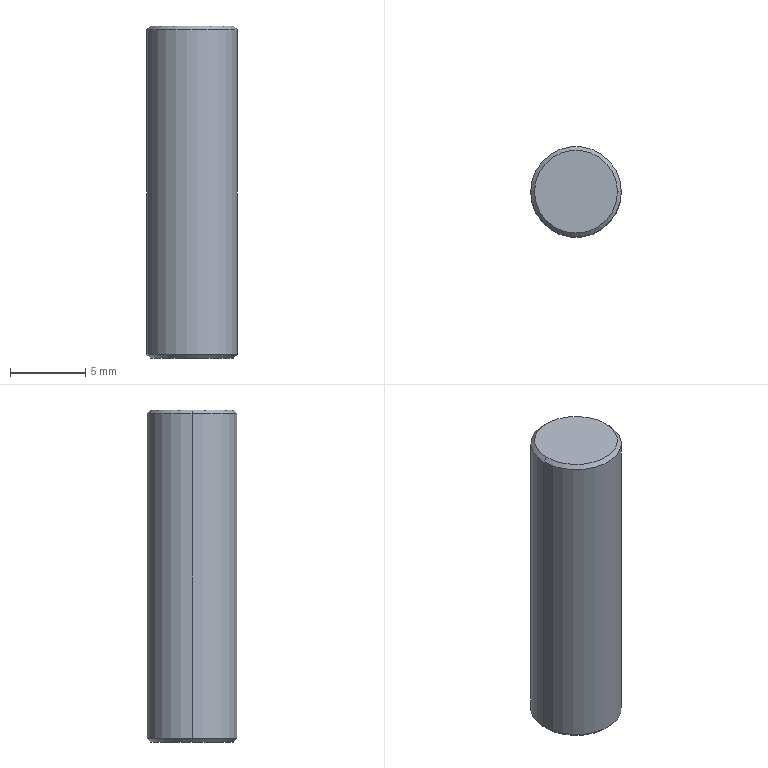Part | STEP file | CHOT CAI | 1 solid | 8 faces | box 6 x 6 x 22 mm | volume 620.89 mm3 | cone 4 | cylinder 2 | plane 2 | commonest cylinder face diameters 6 x2
STEP:
#1=CARTESIAN_POINT('',(0.,0.,0.));
#2=DIRECTION('',(0.,0.,1.));
#3=DIRECTION('',(1.,0.,0.));
#4=AXIS2_PLACEMENT_3D('',#1,#2,#3);
#5=CARTESIAN_POINT('',(3.,0.,0.25));
#6=VERTEX_POINT('',#5);
#7=CARTESIAN_POINT('',(-3.,0.,0.25));
#8=VERTEX_POINT('',#7);
#9=CARTESIAN_POINT('',(0.,0.,0.25));
#10=DIRECTION('',(0.,0.,1.));
#11=DIRECTION('',(1.,0.,0.));
#12=AXIS2_PLACEMENT_3D('',#9,#10,#11);
#13=CIRCLE('',#12,3.);
#14=CARTESIAN_POINT('',(0.,0.,0.));
#15=DIRECTION('',(0.,0.,1.));
#16=DIRECTION('',(1.,0.,0.));
#17=AXIS2_PLACEMENT_3D('',#14,#15,#16);
#18=CYLINDRICAL_SURFACE('',#17,3.);
#19=CARTESIAN_POINT('',(0.,0.25));
#20=DIRECTION('',(1.,0.));
#21=VECTOR('',#20,1.);
#22=LINE('',#19,#21);
#23=(GEOMETRIC_REPRESENTATION_CONTEXT(2)PARAMETRIC_REPRESENTATION_CONTEXT()REPRESENTATION_CONTEXT('',''));
#24=DEFINITIONAL_REPRESENTATION('',(#22),#23);
#25=PCURVE('',#18,#24);
#26=CARTESIAN_POINT('',(0.,0.,0.25));
#27=DIRECTION('',(0.,0.,1.));
#28=DIRECTION('',(1.,0.,0.));
#29=AXIS2_PLACEMENT_3D('',#26,#27,#28);
#30=CONICAL_SURFACE('',#29,3.,0.7854);
#31=CARTESIAN_POINT('',(0.,0.));
#32=DIRECTION('',(1.,0.));
#33=VECTOR('',#32,1.);
#34=LINE('',#31,#33);
#35=(GEOMETRIC_REPRESENTATION_CONTEXT(2)PARAMETRIC_REPRESENTATION_CONTEXT()REPRESENTATION_CONTEXT('',''));
#36=DEFINITIONAL_REPRESENTATION('',(#34),#35);
#37=PCURVE('',#30,#36);
#38=SURFACE_CURVE('',#13,(#25,#37),.PCURVE_S1.);
#39=EDGE_CURVE('',#6,#8,#38,.T.);
#40=ORIENTED_EDGE('',*,*,#39,.T.);
#41=CARTESIAN_POINT('',(-3.,0.,21.75));
#42=VERTEX_POINT('',#41);
#43=CARTESIAN_POINT('',(-3.,0.,0.));
#44=DIRECTION('',(0.,0.,1.));
#45=VECTOR('',#44,1.);
#46=LINE('',#43,#45);
#47=CARTESIAN_POINT('',(3.142,0.));
#48=DIRECTION('',(0.,1.));
#49=VECTOR('',#48,1.);
#50=LINE('',#47,#49);
#51=(GEOMETRIC_REPRESENTATION_CONTEXT(2)PARAMETRIC_REPRESENTATION_CONTEXT()REPRESENTATION_CONTEXT('',''));
#52=DEFINITIONAL_REPRESENTATION('',(#50),#51);
#53=PCURVE('',#18,#52);
#54=CARTESIAN_POINT('',(0.,0.,0.));
#55=DIRECTION('',(0.,0.,1.));
#56=DIRECTION('',(1.,0.,0.));
#57=AXIS2_PLACEMENT_3D('',#54,#55,#56);
#58=CYLINDRICAL_SURFACE('',#57,3.);
#59=CARTESIAN_POINT('',(3.142,0.));
#60=DIRECTION('',(0.,1.));
#61=VECTOR('',#60,1.);
#62=LINE('',#59,#61);
#63=(GEOMETRIC_REPRESENTATION_CONTEXT(2)PARAMETRIC_REPRESENTATION_CONTEXT()REPRESENTATION_CONTEXT('',''));
#64=DEFINITIONAL_REPRESENTATION('',(#62),#63);
#65=PCURVE('',#58,#64);
#66=SURFACE_CURVE('',#46,(#53,#65),.PCURVE_S1.);
#67=EDGE_CURVE('',#8,#42,#66,.T.);
#68=ORIENTED_EDGE('',*,*,#67,.T.);
#69=CARTESIAN_POINT('',(3.,0.,21.75));
#70=VERTEX_POINT('',#69);
#71=CARTESIAN_POINT('',(0.,0.,21.75));
#72=DIRECTION('',(0.,0.,-1.));
#73=DIRECTION('',(1.,0.,0.));
#74=AXIS2_PLACEMENT_3D('',#71,#72,#73);
#75=CIRCLE('',#74,3.);
#76=CARTESIAN_POINT('',(6.283,21.75));
#77=DIRECTION('',(-1.,0.));
#78=VECTOR('',#77,1.);
#79=LINE('',#76,#78);
#80=(GEOMETRIC_REPRESENTATION_CONTEXT(2)PARAMETRIC_REPRESENTATION_CONTEXT()REPRESENTATION_CONTEXT('',''));
#81=DEFINITIONAL_REPRESENTATION('',(#79),#80);
#82=PCURVE('',#18,#81);
#83=CARTESIAN_POINT('',(0.,0.,21.75));
#84=DIRECTION('',(0.,0.,-1.));
#85=DIRECTION('',(-1.,0.,0.));
#86=AXIS2_PLACEMENT_3D('',#83,#84,#85);
#87=CONICAL_SURFACE('',#86,3.,0.7854);
#88=CARTESIAN_POINT('',(-3.142,0.));
#89=DIRECTION('',(1.,0.));
#90=VECTOR('',#89,1.);
#91=LINE('',#88,#90);
#92=(GEOMETRIC_REPRESENTATION_CONTEXT(2)PARAMETRIC_REPRESENTATION_CONTEXT()REPRESENTATION_CONTEXT('',''));
#93=DEFINITIONAL_REPRESENTATION('',(#91),#92);
#94=PCURVE('',#87,#93);
#95=SURFACE_CURVE('',#75,(#82,#94),.PCURVE_S1.);
#96=EDGE_CURVE('',#42,#70,#95,.T.);
#97=ORIENTED_EDGE('',*,*,#96,.T.);
#98=CARTESIAN_POINT('',(3.,0.,0.));
#99=DIRECTION('',(0.,0.,1.));
#100=VECTOR('',#99,1.);
#101=LINE('',#98,#100);
#102=CARTESIAN_POINT('',(0.,0.));
#103=DIRECTION('',(0.,1.));
#104=VECTOR('',#103,1.);
#105=LINE('',#102,#104);
#106=(GEOMETRIC_REPRESENTATION_CONTEXT(2)PARAMETRIC_REPRESENTATION_CONTEXT()REPRESENTATION_CONTEXT('',''));
#107=DEFINITIONAL_REPRESENTATION('',(#105),#106);
#108=PCURVE('',#18,#107);
#109=CARTESIAN_POINT('',(6.283,0.));
#110=DIRECTION('',(0.,1.));
#111=VECTOR('',#110,1.);
#112=LINE('',#109,#111);
#113=(GEOMETRIC_REPRESENTATION_CONTEXT(2)PARAMETRIC_REPRESENTATION_CONTEXT()REPRESENTATION_CONTEXT('',''));
#114=DEFINITIONAL_REPRESENTATION('',(#112),#113);
#115=PCURVE('',#58,#114);
#116=SURFACE_CURVE('',#101,(#108,#115),.PCURVE_S1.);
#117=EDGE_CURVE('',#6,#70,#116,.T.);
#118=ORIENTED_EDGE('',*,*,#117,.F.);
#119=EDGE_LOOP('',(#40,#68,#97,#118));
#120=FACE_BOUND('',#119,.T.);
#121=ADVANCED_FACE('',(#120),#18,.T.);
#122=CARTESIAN_POINT('',(2.75,0.,0.));
#123=VERTEX_POINT('',#122);
#124=CARTESIAN_POINT('',(-2.75,0.,0.));
#125=VERTEX_POINT('',#124);
#126=CARTESIAN_POINT('',(0.,0.,0.));
#127=DIRECTION('',(0.,0.,1.));
#128=DIRECTION('',(1.,0.,0.));
#129=AXIS2_PLACEMENT_3D('',#126,#127,#128);
#130=CIRCLE('',#129,2.75);
#131=CARTESIAN_POINT('',(0.,-0.25));
#132=DIRECTION('',(1.,0.));
#133=VECTOR('',#132,1.);
#134=LINE('',#131,#133);
#135=(GEOMETRIC_REPRESENTATION_CONTEXT(2)PARAMETRIC_REPRESENTATION_CONTEXT()REPRESENTATION_CONTEXT('',''));
#136=DEFINITIONAL_REPRESENTATION('',(#134),#135);
#137=PCURVE('',#30,#136);
#138=CARTESIAN_POINT('',(0.,0.,0.));
#139=DIRECTION('',(0.,0.,-1.));
#140=DIRECTION('',(-1.,0.,0.));
#141=AXIS2_PLACEMENT_3D('',#138,#139,#140);
#142=PLANE('',#141);
#143=CARTESIAN_POINT('',(-2.75,0.));
#144=CARTESIAN_POINT('',(-2.75,4.763));
#145=CARTESIAN_POINT('',(1.375,2.382));
#146=CARTESIAN_POINT('',(5.5,0.));
#147=CARTESIAN_POINT('',(1.375,-2.382));
#148=CARTESIAN_POINT('',(-2.75,-4.763));
#149=CARTESIAN_POINT('',(-2.75,0.));
#150=(BOUNDED_CURVE()B_SPLINE_CURVE(2,(#143,#144,#145,#146,#147,#148,#149),.UNSPECIFIED.,.T.,.F.)B_SPLINE_CURVE_WITH_KNOTS((1,2,2,2,2,1),(-2.094,0.,2.094,4.189,6.283,8.378),.UNSPECIFIED.)CURVE()GEOMETRIC_REPRESENTATION_ITEM()RATIONAL_B_SPLINE_CURVE((1.,0.5,1.,0.5,1.,0.5,1.))REPRESENTATION_ITEM(''));
#151=(GEOMETRIC_REPRESENTATION_CONTEXT(2)PARAMETRIC_REPRESENTATION_CONTEXT()REPRESENTATION_CONTEXT('',''));
#152=DEFINITIONAL_REPRESENTATION('',(#150),#151);
#153=PCURVE('',#142,#152);
#154=SURFACE_CURVE('',#130,(#137,#153),.PCURVE_S1.);
#155=EDGE_CURVE('',#123,#125,#154,.T.);
#156=ORIENTED_EDGE('',*,*,#155,.T.);
#157=CARTESIAN_POINT('',(-3.,0.,0.25));
#158=DIRECTION('',(-0.7071,0.,0.7071));
#159=VECTOR('',#158,1.);
#160=LINE('',#157,#159);
#161=CARTESIAN_POINT('',(3.142,0.));
#162=DIRECTION('',(0.,1.));
#163=VECTOR('',#162,1.);
#164=LINE('',#161,#163);
#165=(GEOMETRIC_REPRESENTATION_CONTEXT(2)PARAMETRIC_REPRESENTATION_CONTEXT()REPRESENTATION_CONTEXT('',''));
#166=DEFINITIONAL_REPRESENTATION('',(#164),#165);
#167=PCURVE('',#30,#166);
#168=CARTESIAN_POINT('',(0.,0.,0.25));
#169=DIRECTION('',(0.,0.,1.));
#170=DIRECTION('',(1.,0.,0.));
#171=AXIS2_PLACEMENT_3D('',#168,#169,#170);
#172=CONICAL_SURFACE('',#171,3.,0.7854);
#173=CARTESIAN_POINT('',(3.142,0.));
#174=DIRECTION('',(0.,1.));
#175=VECTOR('',#174,1.);
#176=LINE('',#173,#175);
#177=(GEOMETRIC_REPRESENTATION_CONTEXT(2)PARAMETRIC_REPRESENTATION_CONTEXT()REPRESENTATION_CONTEXT('',''));
#178=DEFINITIONAL_REPRESENTATION('',(#176),#177);
#179=PCURVE('',#172,#178);
#180=SURFACE_CURVE('',#160,(#167,#179),.PCURVE_S1.);
#181=EDGE_CURVE('',#125,#8,#180,.T.);
#182=ORIENTED_EDGE('',*,*,#181,.T.);
#183=ORIENTED_EDGE('',*,*,#39,.F.);
#184=CARTESIAN_POINT('',(3.,0.,0.25));
#185=DIRECTION('',(0.7071,0.,0.7071));
#186=VECTOR('',#185,1.);
#187=LINE('',#184,#186);
#188=CARTESIAN_POINT('',(0.,0.));
#189=DIRECTION('',(0.,1.));
#190=VECTOR('',#189,1.);
#191=LINE('',#188,#190);
#192=(GEOMETRIC_REPRESENTATION_CONTEXT(2)PARAMETRIC_REPRESENTATION_CONTEXT()REPRESENTATION_CONTEXT('',''));
#193=DEFINITIONAL_REPRESENTATION('',(#191),#192);
#194=PCURVE('',#30,#193);
#195=CARTESIAN_POINT('',(6.283,0.));
#196=DIRECTION('',(0.,1.));
#197=VECTOR('',#196,1.);
#198=LINE('',#195,#197);
#199=(GEOMETRIC_REPRESENTATION_CONTEXT(2)PARAMETRIC_REPRESENTATION_CONTEXT()REPRESENTATION_CONTEXT('',''));
#200=DEFINITIONAL_REPRESENTATION('',(#198),#199);
#201=PCURVE('',#172,#200);
#202=SURFACE_CURVE('',#187,(#194,#201),.PCURVE_S1.);
#203=EDGE_CURVE('',#123,#6,#202,.T.);
#204=ORIENTED_EDGE('',*,*,#203,.F.);
#205=EDGE_LOOP('',(#156,#182,#183,#204));
#206=FACE_BOUND('',#205,.T.);
#207=ADVANCED_FACE('',(#206),#30,.T.);
#208=CARTESIAN_POINT('',(-2.75,0.,22.));
#209=VERTEX_POINT('',#208);
#210=CARTESIAN_POINT('',(2.75,0.,22.));
#211=VERTEX_POINT('',#210);
#212=CARTESIAN_POINT('',(0.,0.,22.));
#213=DIRECTION('',(0.,0.,-1.));
#214=DIRECTION('',(-1.,0.,0.));
#215=AXIS2_PLACEMENT_3D('',#212,#213,#214);
#216=CIRCLE('',#215,2.75);
#217=CARTESIAN_POINT('',(0.,-0.25));
#218=DIRECTION('',(1.,0.));
#219=VECTOR('',#218,1.);
#220=LINE('',#217,#219);
#221=(GEOMETRIC_REPRESENTATION_CONTEXT(2)PARAMETRIC_REPRESENTATION_CONTEXT()REPRESENTATION_CONTEXT('',''));
#222=DEFINITIONAL_REPRESENTATION('',(#220),#221);
#223=PCURVE('',#87,#222);
#224=CARTESIAN_POINT('',(0.,0.,22.));
#225=DIRECTION('',(0.,0.,-1.));
#226=DIRECTION('',(-1.,0.,0.));
#227=AXIS2_PLACEMENT_3D('',#224,#225,#226);
#228=PLANE('',#227);
#229=CARTESIAN_POINT('',(0.,0.));
#230=DIRECTION('',(1.,0.));
#231=AXIS2_PLACEMENT_2D('',#229,#230);
#232=CIRCLE('',#231,2.75);
#233=(GEOMETRIC_REPRESENTATION_CONTEXT(2)PARAMETRIC_REPRESENTATION_CONTEXT()REPRESENTATION_CONTEXT('',''));
#234=DEFINITIONAL_REPRESENTATION('',(#232),#233);
#235=PCURVE('',#228,#234);
#236=SURFACE_CURVE('',#216,(#223,#235),.PCURVE_S1.);
#237=EDGE_CURVE('',#209,#211,#236,.T.);
#238=ORIENTED_EDGE('',*,*,#237,.T.);
#239=CARTESIAN_POINT('',(3.,0.,21.75));
#240=DIRECTION('',(0.7071,0.,-0.7071));
#241=VECTOR('',#240,1.);
#242=LINE('',#239,#241);
#243=CARTESIAN_POINT('',(3.142,0.));
#244=DIRECTION('',(0.,1.));
#245=VECTOR('',#244,1.);
#246=LINE('',#243,#245);
#247=(GEOMETRIC_REPRESENTATION_CONTEXT(2)PARAMETRIC_REPRESENTATION_CONTEXT()REPRESENTATION_CONTEXT('',''));
#248=DEFINITIONAL_REPRESENTATION('',(#246),#247);
#249=PCURVE('',#87,#248);
#250=CARTESIAN_POINT('',(0.,0.,21.75));
#251=DIRECTION('',(0.,0.,-1.));
#252=DIRECTION('',(-1.,0.,0.));
#253=AXIS2_PLACEMENT_3D('',#250,#251,#252);
#254=CONICAL_SURFACE('',#253,3.,0.7854);
#255=CARTESIAN_POINT('',(3.142,0.));
#256=DIRECTION('',(0.,1.));
#257=VECTOR('',#256,1.);
#258=LINE('',#255,#257);
#259=(GEOMETRIC_REPRESENTATION_CONTEXT(2)PARAMETRIC_REPRESENTATION_CONTEXT()REPRESENTATION_CONTEXT('',''));
#260=DEFINITIONAL_REPRESENTATION('',(#258),#259);
#261=PCURVE('',#254,#260);
#262=SURFACE_CURVE('',#242,(#249,#261),.PCURVE_S1.);
#263=EDGE_CURVE('',#211,#70,#262,.T.);
#264=ORIENTED_EDGE('',*,*,#263,.T.);
#265=ORIENTED_EDGE('',*,*,#96,.F.);
#266=CARTESIAN_POINT('',(-3.,0.,21.75));
#267=DIRECTION('',(-0.7071,0.,-0.7071));
#268=VECTOR('',#267,1.);
#269=LINE('',#266,#268);
#270=CARTESIAN_POINT('',(0.,0.));
#271=DIRECTION('',(0.,1.));
#272=VECTOR('',#271,1.);
#273=LINE('',#270,#272);
#274=(GEOMETRIC_REPRESENTATION_CONTEXT(2)PARAMETRIC_REPRESENTATION_CONTEXT()REPRESENTATION_CONTEXT('',''));
#275=DEFINITIONAL_REPRESENTATION('',(#273),#274);
#276=PCURVE('',#87,#275);
#277=CARTESIAN_POINT('',(6.283,0.));
#278=DIRECTION('',(0.,1.));
#279=VECTOR('',#278,1.);
#280=LINE('',#277,#279);
#281=(GEOMETRIC_REPRESENTATION_CONTEXT(2)PARAMETRIC_REPRESENTATION_CONTEXT()REPRESENTATION_CONTEXT('',''));
#282=DEFINITIONAL_REPRESENTATION('',(#280),#281);
#283=PCURVE('',#254,#282);
#284=SURFACE_CURVE('',#269,(#276,#283),.PCURVE_S1.);
#285=EDGE_CURVE('',#209,#42,#284,.T.);
#286=ORIENTED_EDGE('',*,*,#285,.F.);
#287=EDGE_LOOP('',(#238,#264,#265,#286));
#288=FACE_BOUND('',#287,.T.);
#289=ADVANCED_FACE('',(#288),#87,.T.);
#290=ORIENTED_EDGE('',*,*,#67,.F.);
#291=CARTESIAN_POINT('',(0.,0.,0.25));
#292=DIRECTION('',(0.,0.,1.));
#293=DIRECTION('',(1.,0.,0.));
#294=AXIS2_PLACEMENT_3D('',#291,#292,#293);
#295=CIRCLE('',#294,3.);
#296=CARTESIAN_POINT('',(0.,0.25));
#297=DIRECTION('',(1.,0.));
#298=VECTOR('',#297,1.);
#299=LINE('',#296,#298);
#300=(GEOMETRIC_REPRESENTATION_CONTEXT(2)PARAMETRIC_REPRESENTATION_CONTEXT()REPRESENTATION_CONTEXT('',''));
#301=DEFINITIONAL_REPRESENTATION('',(#299),#300);
#302=PCURVE('',#58,#301);
#303=CARTESIAN_POINT('',(0.,0.));
#304=DIRECTION('',(1.,0.));
#305=VECTOR('',#304,1.);
#306=LINE('',#303,#305);
#307=(GEOMETRIC_REPRESENTATION_CONTEXT(2)PARAMETRIC_REPRESENTATION_CONTEXT()REPRESENTATION_CONTEXT('',''));
#308=DEFINITIONAL_REPRESENTATION('',(#306),#307);
#309=PCURVE('',#172,#308);
#310=SURFACE_CURVE('',#295,(#302,#309),.PCURVE_S1.);
#311=EDGE_CURVE('',#8,#6,#310,.T.);
#312=ORIENTED_EDGE('',*,*,#311,.T.);
#313=ORIENTED_EDGE('',*,*,#117,.T.);
#314=CARTESIAN_POINT('',(0.,0.,21.75));
#315=DIRECTION('',(0.,0.,-1.));
#316=DIRECTION('',(1.,0.,0.));
#317=AXIS2_PLACEMENT_3D('',#314,#315,#316);
#318=CIRCLE('',#317,3.);
#319=CARTESIAN_POINT('',(6.283,21.75));
#320=DIRECTION('',(-1.,0.));
#321=VECTOR('',#320,1.);
#322=LINE('',#319,#321);
#323=(GEOMETRIC_REPRESENTATION_CONTEXT(2)PARAMETRIC_REPRESENTATION_CONTEXT()REPRESENTATION_CONTEXT('',''));
#324=DEFINITIONAL_REPRESENTATION('',(#322),#323);
#325=PCURVE('',#58,#324);
#326=CARTESIAN_POINT('',(3.142,0.));
#327=DIRECTION('',(1.,0.));
#328=VECTOR('',#327,1.);
#329=LINE('',#326,#328);
#330=(GEOMETRIC_REPRESENTATION_CONTEXT(2)PARAMETRIC_REPRESENTATION_CONTEXT()REPRESENTATION_CONTEXT('',''));
#331=DEFINITIONAL_REPRESENTATION('',(#329),#330);
#332=PCURVE('',#254,#331);
#333=SURFACE_CURVE('',#318,(#325,#332),.PCURVE_S1.);
#334=EDGE_CURVE('',#70,#42,#333,.T.);
#335=ORIENTED_EDGE('',*,*,#334,.T.);
#336=EDGE_LOOP('',(#290,#312,#313,#335));
#337=FACE_BOUND('',#336,.T.);
#338=ADVANCED_FACE('',(#337),#58,.T.);
#339=ORIENTED_EDGE('',*,*,#181,.F.);
#340=CARTESIAN_POINT('',(0.,0.,0.));
#341=DIRECTION('',(0.,0.,1.));
#342=DIRECTION('',(1.,0.,0.));
#343=AXIS2_PLACEMENT_3D('',#340,#341,#342);
#344=CIRCLE('',#343,2.75);
#345=CARTESIAN_POINT('',(0.,-0.25));
#346=DIRECTION('',(1.,0.));
#347=VECTOR('',#346,1.);
#348=LINE('',#345,#347);
#349=(GEOMETRIC_REPRESENTATION_CONTEXT(2)PARAMETRIC_REPRESENTATION_CONTEXT()REPRESENTATION_CONTEXT('',''));
#350=DEFINITIONAL_REPRESENTATION('',(#348),#349);
#351=PCURVE('',#172,#350);
#352=CARTESIAN_POINT('',(-2.75,0.));
#353=CARTESIAN_POINT('',(-2.75,4.763));
#354=CARTESIAN_POINT('',(1.375,2.382));
#355=CARTESIAN_POINT('',(5.5,0.));
#356=CARTESIAN_POINT('',(1.375,-2.382));
#357=CARTESIAN_POINT('',(-2.75,-4.763));
#358=CARTESIAN_POINT('',(-2.75,0.));
#359=(BOUNDED_CURVE()B_SPLINE_CURVE(2,(#352,#353,#354,#355,#356,#357,#358),.UNSPECIFIED.,.T.,.F.)B_SPLINE_CURVE_WITH_KNOTS((1,2,2,2,2,1),(-2.094,0.,2.094,4.189,6.283,8.378),.UNSPECIFIED.)CURVE()GEOMETRIC_REPRESENTATION_ITEM()RATIONAL_B_SPLINE_CURVE((1.,0.5,1.,0.5,1.,0.5,1.))REPRESENTATION_ITEM(''));
#360=(GEOMETRIC_REPRESENTATION_CONTEXT(2)PARAMETRIC_REPRESENTATION_CONTEXT()REPRESENTATION_CONTEXT('',''));
#361=DEFINITIONAL_REPRESENTATION('',(#359),#360);
#362=PCURVE('',#142,#361);
#363=SURFACE_CURVE('',#344,(#351,#362),.PCURVE_S1.);
#364=EDGE_CURVE('',#125,#123,#363,.T.);
#365=ORIENTED_EDGE('',*,*,#364,.T.);
#366=ORIENTED_EDGE('',*,*,#203,.T.);
#367=ORIENTED_EDGE('',*,*,#311,.F.);
#368=EDGE_LOOP('',(#339,#365,#366,#367));
#369=FACE_BOUND('',#368,.T.);
#370=ADVANCED_FACE('',(#369),#172,.T.);
#371=ORIENTED_EDGE('',*,*,#263,.F.);
#372=CARTESIAN_POINT('',(0.,0.,22.));
#373=DIRECTION('',(0.,0.,-1.));
#374=DIRECTION('',(-1.,0.,0.));
#375=AXIS2_PLACEMENT_3D('',#372,#373,#374);
#376=CIRCLE('',#375,2.75);
#377=CARTESIAN_POINT('',(0.,-0.25));
#378=DIRECTION('',(1.,0.));
#379=VECTOR('',#378,1.);
#380=LINE('',#377,#379);
#381=(GEOMETRIC_REPRESENTATION_CONTEXT(2)PARAMETRIC_REPRESENTATION_CONTEXT()REPRESENTATION_CONTEXT('',''));
#382=DEFINITIONAL_REPRESENTATION('',(#380),#381);
#383=PCURVE('',#254,#382);
#384=CARTESIAN_POINT('',(0.,0.));
#385=DIRECTION('',(1.,0.));
#386=AXIS2_PLACEMENT_2D('',#384,#385);
#387=CIRCLE('',#386,2.75);
#388=(GEOMETRIC_REPRESENTATION_CONTEXT(2)PARAMETRIC_REPRESENTATION_CONTEXT()REPRESENTATION_CONTEXT('',''));
#389=DEFINITIONAL_REPRESENTATION('',(#387),#388);
#390=PCURVE('',#228,#389);
#391=SURFACE_CURVE('',#376,(#383,#390),.PCURVE_S1.);
#392=EDGE_CURVE('',#211,#209,#391,.T.);
#393=ORIENTED_EDGE('',*,*,#392,.T.);
#394=ORIENTED_EDGE('',*,*,#285,.T.);
#395=ORIENTED_EDGE('',*,*,#334,.F.);
#396=EDGE_LOOP('',(#371,#393,#394,#395));
#397=FACE_BOUND('',#396,.T.);
#398=ADVANCED_FACE('',(#397),#254,.T.);
#399=ORIENTED_EDGE('',*,*,#155,.F.);
#400=ORIENTED_EDGE('',*,*,#364,.F.);
#401=EDGE_LOOP('',(#399,#400));
#402=FACE_BOUND('',#401,.T.);
#403=ADVANCED_FACE('',(#402),#142,.T.);
#404=ORIENTED_EDGE('',*,*,#237,.F.);
#405=ORIENTED_EDGE('',*,*,#392,.F.);
#406=EDGE_LOOP('',(#404,#405));
#407=FACE_BOUND('',#406,.T.);
#408=ADVANCED_FACE('',(#407),#228,.F.);
#409=CLOSED_SHELL('',(#121,#207,#289,#338,#370,#398,#403,#408));
#410=MANIFOLD_SOLID_BREP('',#409);
#411=(LENGTH_UNIT()NAMED_UNIT(*)SI_UNIT(.MILLI.,.METRE.));
#412=UNCERTAINTY_MEASURE_WITH_UNIT(LENGTH_MEASURE(0.0000001),#411,'','');
#413=(NAMED_UNIT(*)PLANE_ANGLE_UNIT()SI_UNIT($,.RADIAN.));
#414=(NAMED_UNIT(*)SI_UNIT($,.STERADIAN.)SOLID_ANGLE_UNIT());
#415=(GEOMETRIC_REPRESENTATION_CONTEXT(3)GLOBAL_UNCERTAINTY_ASSIGNED_CONTEXT((#412))GLOBAL_UNIT_ASSIGNED_CONTEXT((#411,#413,#414))REPRESENTATION_CONTEXT('',''));
#416=ADVANCED_BREP_SHAPE_REPRESENTATION('',(#4,#410),#415);